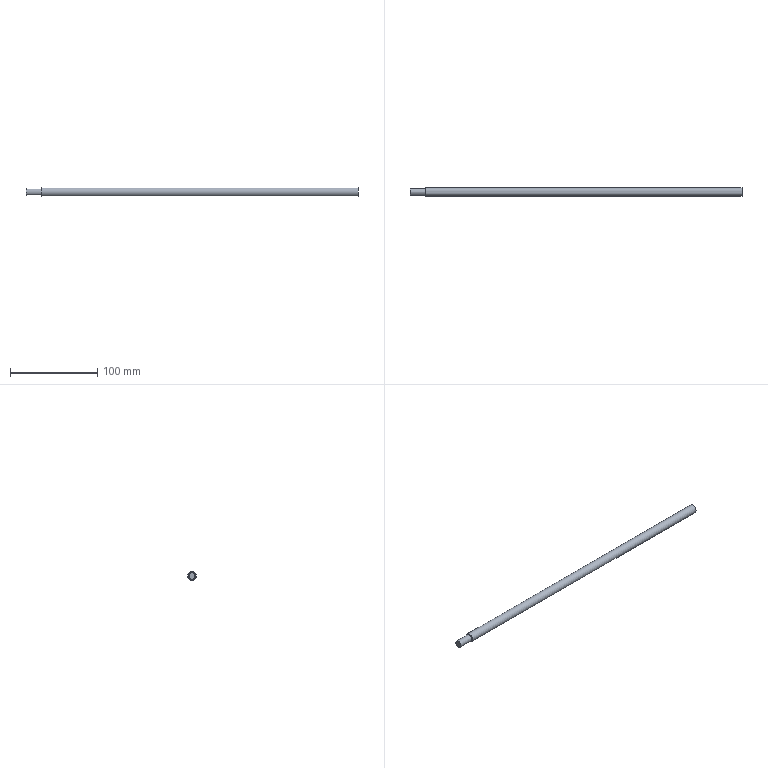Part | STEP file | SN10_015_003_GUIA | 1 solid | 6 faces | box 380 x 10 x 10 mm | volume 29333 mm3 | plane 3 | cylinder 2 | cone 1 | commonest cylinder face diameters 8 x1 10 x1
STEP:
#1=CARTESIAN_POINT('',(0.,0.,0.));
#2=DIRECTION('',(0.,0.,1.));
#3=DIRECTION('',(1.,0.,0.));
#4=AXIS2_PLACEMENT_3D('',#1,#2,#3);
#5=CARTESIAN_POINT('',(5523.342,-1740.101,67.25));
#6=VERTEX_POINT('',#5);
#7=CARTESIAN_POINT('',(5523.342,-1745.101,67.25));
#8=DIRECTION('',(-1.,0.,0.));
#9=DIRECTION('',(0.,1.,0.));
#10=AXIS2_PLACEMENT_3D('',#7,#8,#9);
#11=CIRCLE('',#10,5.);
#12=CARTESIAN_POINT('',(5523.342,0.,0.));
#13=DIRECTION('',(-1.,0.,0.));
#14=DIRECTION('',(0.,0.,1.));
#15=AXIS2_PLACEMENT_3D('',#12,#13,#14);
#16=PLANE('',#15);
#17=CARTESIAN_POINT('',(67.25,-1745.101));
#18=DIRECTION('',(0.,1.));
#19=AXIS2_PLACEMENT_2D('',#17,#18);
#20=CIRCLE('',#19,5.);
#21=(GEOMETRIC_REPRESENTATION_CONTEXT(2)PARAMETRIC_REPRESENTATION_CONTEXT()REPRESENTATION_CONTEXT('',''));
#22=DEFINITIONAL_REPRESENTATION('',(#20),#21);
#23=PCURVE('',#16,#22);
#24=CARTESIAN_POINT('',(5695.342,-1745.101,67.25));
#25=DIRECTION('',(-1.,0.,0.));
#26=DIRECTION('',(0.,-1.,0.));
#27=AXIS2_PLACEMENT_3D('',#24,#25,#26);
#28=CYLINDRICAL_SURFACE('',#27,5.);
#29=CARTESIAN_POINT('',(3.142,172.));
#30=DIRECTION('',(1.,0.));
#31=VECTOR('',#30,1.);
#32=LINE('',#29,#31);
#33=(GEOMETRIC_REPRESENTATION_CONTEXT(2)PARAMETRIC_REPRESENTATION_CONTEXT()REPRESENTATION_CONTEXT('',''));
#34=DEFINITIONAL_REPRESENTATION('',(#32),#33);
#35=PCURVE('',#28,#34);
#36=SURFACE_CURVE('',#11,(#23,#35),.PCURVE_S1.);
#37=EDGE_CURVE('',#6,#6,#36,.T.);
#38=ORIENTED_EDGE('',*,*,#37,.T.);
#39=EDGE_LOOP('',(#38));
#40=FACE_BOUND('',#39,.T.);
#41=CARTESIAN_POINT('',(5523.342,-1741.101,67.25));
#42=VERTEX_POINT('',#41);
#43=CARTESIAN_POINT('',(5523.342,-1745.101,67.25));
#44=DIRECTION('',(-1.,0.,0.));
#45=DIRECTION('',(0.,1.,0.));
#46=AXIS2_PLACEMENT_3D('',#43,#44,#45);
#47=CIRCLE('',#46,4.);
#48=CARTESIAN_POINT('',(67.25,-1745.101));
#49=DIRECTION('',(0.,1.));
#50=AXIS2_PLACEMENT_2D('',#48,#49);
#51=CIRCLE('',#50,4.);
#52=(GEOMETRIC_REPRESENTATION_CONTEXT(2)PARAMETRIC_REPRESENTATION_CONTEXT()REPRESENTATION_CONTEXT('',''));
#53=DEFINITIONAL_REPRESENTATION('',(#51),#52);
#54=PCURVE('',#16,#53);
#55=CARTESIAN_POINT('',(5513.682,-1745.101,67.25));
#56=DIRECTION('',(-1.,0.,0.));
#57=DIRECTION('',(0.,-1.,0.));
#58=AXIS2_PLACEMENT_3D('',#55,#56,#57);
#59=CYLINDRICAL_SURFACE('',#58,4.);
#60=CARTESIAN_POINT('',(3.142,-9.66));
#61=DIRECTION('',(1.,0.));
#62=VECTOR('',#61,1.);
#63=LINE('',#60,#62);
#64=(GEOMETRIC_REPRESENTATION_CONTEXT(2)PARAMETRIC_REPRESENTATION_CONTEXT()REPRESENTATION_CONTEXT('',''));
#65=DEFINITIONAL_REPRESENTATION('',(#63),#64);
#66=PCURVE('',#59,#65);
#67=SURFACE_CURVE('',#47,(#54,#66),.PCURVE_S1.);
#68=EDGE_CURVE('',#42,#42,#67,.T.);
#69=ORIENTED_EDGE('',*,*,#68,.F.);
#70=EDGE_LOOP('',(#69));
#71=FACE_BOUND('',#70,.T.);
#72=ADVANCED_FACE('',(#40,#71),#16,.T.);
#73=ORIENTED_EDGE('',*,*,#37,.F.);
#74=CARTESIAN_POINT('',(5885.342,-1740.101,67.25));
#75=VERTEX_POINT('',#74);
#76=CARTESIAN_POINT('',(5885.342,-1740.101,67.25));
#77=CARTESIAN_POINT('',(5523.342,-1740.101,67.25));
#78=B_SPLINE_CURVE_WITH_KNOTS('',1,(#76,#77),.UNSPECIFIED.,.F.,.F.,(2,2),(-190.,172.),.PIECEWISE_BEZIER_KNOTS.);
#79=CARTESIAN_POINT('',(3.142,0.));
#80=DIRECTION('',(0.,1.));
#81=VECTOR('',#80,1.);
#82=LINE('',#79,#81);
#83=(GEOMETRIC_REPRESENTATION_CONTEXT(2)PARAMETRIC_REPRESENTATION_CONTEXT()REPRESENTATION_CONTEXT('',''));
#84=DEFINITIONAL_REPRESENTATION('',(#82),#83);
#85=PCURVE('',#28,#84);
#86=CARTESIAN_POINT('',(9.425,0.));
#87=DIRECTION('',(0.,1.));
#88=VECTOR('',#87,1.);
#89=LINE('',#86,#88);
#90=(GEOMETRIC_REPRESENTATION_CONTEXT(2)PARAMETRIC_REPRESENTATION_CONTEXT()REPRESENTATION_CONTEXT('',''));
#91=DEFINITIONAL_REPRESENTATION('',(#89),#90);
#92=PCURVE('',#28,#91);
#93=SEAM_CURVE('',#78,(#85,#92),.PCURVE_S1.);
#94=EDGE_CURVE('',#75,#6,#93,.T.);
#95=ORIENTED_EDGE('',*,*,#94,.F.);
#96=CARTESIAN_POINT('',(5885.342,-1745.101,67.25));
#97=DIRECTION('',(-1.,0.,0.));
#98=DIRECTION('',(0.,1.,0.));
#99=AXIS2_PLACEMENT_3D('',#96,#97,#98);
#100=CIRCLE('',#99,5.);
#101=CARTESIAN_POINT('',(3.142,-190.));
#102=DIRECTION('',(1.,0.));
#103=VECTOR('',#102,1.);
#104=LINE('',#101,#103);
#105=(GEOMETRIC_REPRESENTATION_CONTEXT(2)PARAMETRIC_REPRESENTATION_CONTEXT()REPRESENTATION_CONTEXT('',''));
#106=DEFINITIONAL_REPRESENTATION('',(#104),#105);
#107=PCURVE('',#28,#106);
#108=CARTESIAN_POINT('',(5885.342,0.,0.));
#109=DIRECTION('',(-1.,0.,0.));
#110=DIRECTION('',(0.,0.,1.));
#111=AXIS2_PLACEMENT_3D('',#108,#109,#110);
#112=PLANE('',#111);
#113=CARTESIAN_POINT('',(67.25,-1745.101));
#114=DIRECTION('',(0.,1.));
#115=AXIS2_PLACEMENT_2D('',#113,#114);
#116=CIRCLE('',#115,5.);
#117=(GEOMETRIC_REPRESENTATION_CONTEXT(2)PARAMETRIC_REPRESENTATION_CONTEXT()REPRESENTATION_CONTEXT('',''));
#118=DEFINITIONAL_REPRESENTATION('',(#116),#117);
#119=PCURVE('',#112,#118);
#120=SURFACE_CURVE('',#100,(#107,#119),.PCURVE_S1.);
#121=EDGE_CURVE('',#75,#75,#120,.T.);
#122=ORIENTED_EDGE('',*,*,#121,.T.);
#123=ORIENTED_EDGE('',*,*,#94,.T.);
#124=EDGE_LOOP('',(#73,#95,#122,#123));
#125=FACE_BOUND('',#124,.T.);
#126=ADVANCED_FACE('',(#125),#28,.T.);
#127=ORIENTED_EDGE('',*,*,#121,.F.);
#128=EDGE_LOOP('',(#127));
#129=FACE_BOUND('',#128,.T.);
#130=ADVANCED_FACE('',(#129),#112,.F.);
#131=CARTESIAN_POINT('',(5505.342,-1748.601,67.25));
#132=VERTEX_POINT('',#131);
#133=CARTESIAN_POINT('',(5505.342,-1741.601,67.25));
#134=VERTEX_POINT('',#133);
#135=CARTESIAN_POINT('',(5505.342,-1745.101,67.25));
#136=DIRECTION('',(-1.,0.,0.));
#137=DIRECTION('',(0.,1.,0.));
#138=AXIS2_PLACEMENT_3D('',#135,#136,#137);
#139=CIRCLE('',#138,3.5);
#140=CARTESIAN_POINT('',(5505.342,0.,0.));
#141=DIRECTION('',(-1.,0.,0.));
#142=DIRECTION('',(0.,0.,1.));
#143=AXIS2_PLACEMENT_3D('',#140,#141,#142);
#144=PLANE('',#143);
#145=CARTESIAN_POINT('',(67.25,-1745.101));
#146=DIRECTION('',(0.,1.));
#147=AXIS2_PLACEMENT_2D('',#145,#146);
#148=CIRCLE('',#147,3.5);
#149=(GEOMETRIC_REPRESENTATION_CONTEXT(2)PARAMETRIC_REPRESENTATION_CONTEXT()REPRESENTATION_CONTEXT('',''));
#150=DEFINITIONAL_REPRESENTATION('',(#148),#149);
#151=PCURVE('',#144,#150);
#152=CARTESIAN_POINT('',(5502.842,-1745.101,67.25));
#153=DIRECTION('',(1.,0.,0.));
#154=DIRECTION('',(0.,0.8155,0.5788));
#155=AXIS2_PLACEMENT_3D('',#152,#153,#154);
#156=CONICAL_SURFACE('',#155,1.,0.7854);
#157=CARTESIAN_POINT('',(11.949,2.5));
#158=DIRECTION('',(-1.,0.));
#159=VECTOR('',#158,1.);
#160=LINE('',#157,#159);
#161=(GEOMETRIC_REPRESENTATION_CONTEXT(2)PARAMETRIC_REPRESENTATION_CONTEXT()REPRESENTATION_CONTEXT('',''));
#162=DEFINITIONAL_REPRESENTATION('',(#160),#161);
#163=PCURVE('',#156,#162);
#164=SURFACE_CURVE('',#139,(#151,#163),.PCURVE_S1.);
#165=EDGE_CURVE('',#132,#134,#164,.T.);
#166=ORIENTED_EDGE('',*,*,#165,.T.);
#167=CARTESIAN_POINT('',(5505.342,-1745.101,67.25));
#168=DIRECTION('',(-1.,0.,0.));
#169=DIRECTION('',(0.,1.,0.));
#170=AXIS2_PLACEMENT_3D('',#167,#168,#169);
#171=CIRCLE('',#170,3.5);
#172=CARTESIAN_POINT('',(67.25,-1745.101));
#173=DIRECTION('',(0.,1.));
#174=AXIS2_PLACEMENT_2D('',#172,#173);
#175=CIRCLE('',#174,3.5);
#176=(GEOMETRIC_REPRESENTATION_CONTEXT(2)PARAMETRIC_REPRESENTATION_CONTEXT()REPRESENTATION_CONTEXT('',''));
#177=DEFINITIONAL_REPRESENTATION('',(#175),#176);
#178=PCURVE('',#144,#177);
#179=CARTESIAN_POINT('',(11.949,2.5));
#180=DIRECTION('',(-1.,0.));
#181=VECTOR('',#180,1.);
#182=LINE('',#179,#181);
#183=(GEOMETRIC_REPRESENTATION_CONTEXT(2)PARAMETRIC_REPRESENTATION_CONTEXT()REPRESENTATION_CONTEXT('',''));
#184=DEFINITIONAL_REPRESENTATION('',(#182),#183);
#185=PCURVE('',#156,#184);
#186=SURFACE_CURVE('',#171,(#178,#185),.PCURVE_S1.);
#187=EDGE_CURVE('',#134,#132,#186,.T.);
#188=ORIENTED_EDGE('',*,*,#187,.T.);
#189=EDGE_LOOP('',(#166,#188));
#190=FACE_BOUND('',#189,.T.);
#191=ADVANCED_FACE('',(#190),#144,.T.);
#192=CARTESIAN_POINT('',(5505.842,-1741.101,67.25));
#193=VERTEX_POINT('',#192);
#194=CARTESIAN_POINT('',(5505.842,-1745.101,67.25));
#195=DIRECTION('',(-1.,0.,0.));
#196=DIRECTION('',(0.,1.,0.));
#197=AXIS2_PLACEMENT_3D('',#194,#195,#196);
#198=CIRCLE('',#197,4.);
#199=CARTESIAN_POINT('',(3.142,7.84));
#200=DIRECTION('',(1.,0.));
#201=VECTOR('',#200,1.);
#202=LINE('',#199,#201);
#203=(GEOMETRIC_REPRESENTATION_CONTEXT(2)PARAMETRIC_REPRESENTATION_CONTEXT()REPRESENTATION_CONTEXT('',''));
#204=DEFINITIONAL_REPRESENTATION('',(#202),#203);
#205=PCURVE('',#59,#204);
#206=CARTESIAN_POINT('',(11.949,3.));
#207=DIRECTION('',(-1.,0.));
#208=VECTOR('',#207,1.);
#209=LINE('',#206,#208);
#210=(GEOMETRIC_REPRESENTATION_CONTEXT(2)PARAMETRIC_REPRESENTATION_CONTEXT()REPRESENTATION_CONTEXT('',''));
#211=DEFINITIONAL_REPRESENTATION('',(#209),#210);
#212=PCURVE('',#156,#211);
#213=SURFACE_CURVE('',#198,(#205,#212),.PCURVE_S1.);
#214=EDGE_CURVE('',#193,#193,#213,.T.);
#215=ORIENTED_EDGE('',*,*,#214,.F.);
#216=CARTESIAN_POINT('',(5523.342,-1741.101,67.25));
#217=CARTESIAN_POINT('',(5505.842,-1741.101,67.25));
#218=B_SPLINE_CURVE_WITH_KNOTS('',1,(#216,#217),.UNSPECIFIED.,.F.,.F.,(2,2),(-9.66,7.84),.PIECEWISE_BEZIER_KNOTS.);
#219=CARTESIAN_POINT('',(3.142,0.));
#220=DIRECTION('',(0.,1.));
#221=VECTOR('',#220,1.);
#222=LINE('',#219,#221);
#223=(GEOMETRIC_REPRESENTATION_CONTEXT(2)PARAMETRIC_REPRESENTATION_CONTEXT()REPRESENTATION_CONTEXT('',''));
#224=DEFINITIONAL_REPRESENTATION('',(#222),#223);
#225=PCURVE('',#59,#224);
#226=CARTESIAN_POINT('',(9.425,0.));
#227=DIRECTION('',(0.,1.));
#228=VECTOR('',#227,1.);
#229=LINE('',#226,#228);
#230=(GEOMETRIC_REPRESENTATION_CONTEXT(2)PARAMETRIC_REPRESENTATION_CONTEXT()REPRESENTATION_CONTEXT('',''));
#231=DEFINITIONAL_REPRESENTATION('',(#229),#230);
#232=PCURVE('',#59,#231);
#233=SEAM_CURVE('',#218,(#225,#232),.PCURVE_S1.);
#234=EDGE_CURVE('',#42,#193,#233,.T.);
#235=ORIENTED_EDGE('',*,*,#234,.F.);
#236=ORIENTED_EDGE('',*,*,#68,.T.);
#237=ORIENTED_EDGE('',*,*,#234,.T.);
#238=EDGE_LOOP('',(#215,#235,#236,#237));
#239=FACE_BOUND('',#238,.T.);
#240=ADVANCED_FACE('',(#239),#59,.T.);
#241=ORIENTED_EDGE('',*,*,#187,.F.);
#242=CARTESIAN_POINT('',(5505.342,-1741.601,67.25));
#243=CARTESIAN_POINT('',(5505.842,-1741.101,67.25));
#244=B_SPLINE_CURVE_WITH_KNOTS('',1,(#242,#243),.UNSPECIFIED.,.F.,.F.,(2,2),(3.536,4.243),.PIECEWISE_BEZIER_KNOTS.);
#245=CARTESIAN_POINT('',(11.949,0.));
#246=DIRECTION('',(0.,1.));
#247=VECTOR('',#246,1.);
#248=LINE('',#245,#247);
#249=(GEOMETRIC_REPRESENTATION_CONTEXT(2)PARAMETRIC_REPRESENTATION_CONTEXT()REPRESENTATION_CONTEXT('',''));
#250=DEFINITIONAL_REPRESENTATION('',(#248),#249);
#251=PCURVE('',#156,#250);
#252=CARTESIAN_POINT('',(5.666,0.));
#253=DIRECTION('',(0.,1.));
#254=VECTOR('',#253,1.);
#255=LINE('',#252,#254);
#256=(GEOMETRIC_REPRESENTATION_CONTEXT(2)PARAMETRIC_REPRESENTATION_CONTEXT()REPRESENTATION_CONTEXT('',''));
#257=DEFINITIONAL_REPRESENTATION('',(#255),#256);
#258=PCURVE('',#156,#257);
#259=SEAM_CURVE('',#244,(#251,#258),.PCURVE_S1.);
#260=EDGE_CURVE('',#134,#193,#259,.T.);
#261=ORIENTED_EDGE('',*,*,#260,.T.);
#262=ORIENTED_EDGE('',*,*,#214,.T.);
#263=ORIENTED_EDGE('',*,*,#260,.F.);
#264=ORIENTED_EDGE('',*,*,#165,.F.);
#265=EDGE_LOOP('',(#241,#261,#262,#263,#264));
#266=FACE_BOUND('',#265,.T.);
#267=ADVANCED_FACE('',(#266),#156,.T.);
#268=CLOSED_SHELL('',(#72,#126,#130,#191,#240,#267));
#269=MANIFOLD_SOLID_BREP('',#268);
#270=(LENGTH_UNIT()NAMED_UNIT(*)SI_UNIT(.MILLI.,.METRE.));
#271=UNCERTAINTY_MEASURE_WITH_UNIT(LENGTH_MEASURE(0.000005),#270,'','');
#272=(NAMED_UNIT(*)PLANE_ANGLE_UNIT()SI_UNIT($,.RADIAN.));
#273=(NAMED_UNIT(*)SI_UNIT($,.STERADIAN.)SOLID_ANGLE_UNIT());
#274=(GEOMETRIC_REPRESENTATION_CONTEXT(3)GLOBAL_UNCERTAINTY_ASSIGNED_CONTEXT((#271))GLOBAL_UNIT_ASSIGNED_CONTEXT((#270,#272,#273))REPRESENTATION_CONTEXT('',''));
#275=ADVANCED_BREP_SHAPE_REPRESENTATION('',(#4,#269),#274);